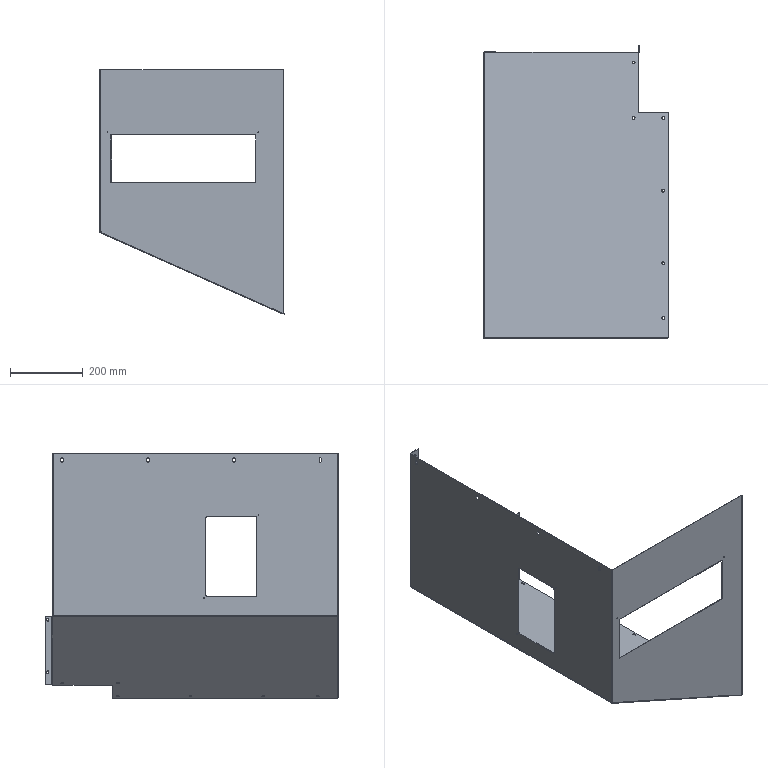Part | NX | features solid 2 | 1 solid | 123 faces | box 507.744 x 806 x 673.765 mm | volume 1565456 mm3 | plane 63 | cylinder 60 | commonest cylinder face diameters 7 x22 8 x12 2.5 x8 5 x6 3 x4 6 x4